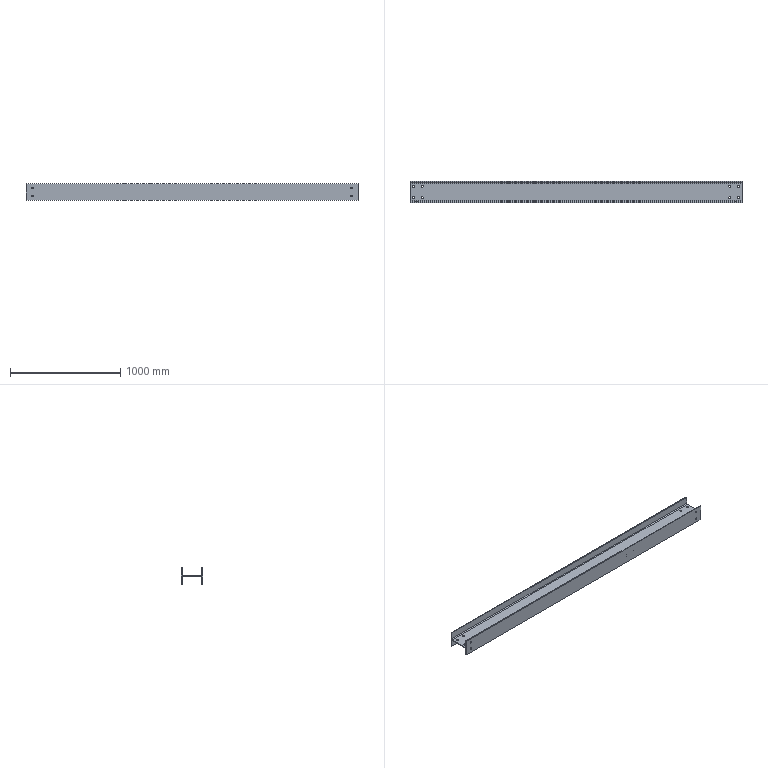Part | STEP file | E3-导轨连接梁1主体_Default<按焊接> | 1 solid | 42 faces | box 3006 x 194 x 150 mm | volume 11435709 mm3 | cylinder 28 | plane 14 | commonest cylinder face diameters 19 x16 15 x8 16 x4